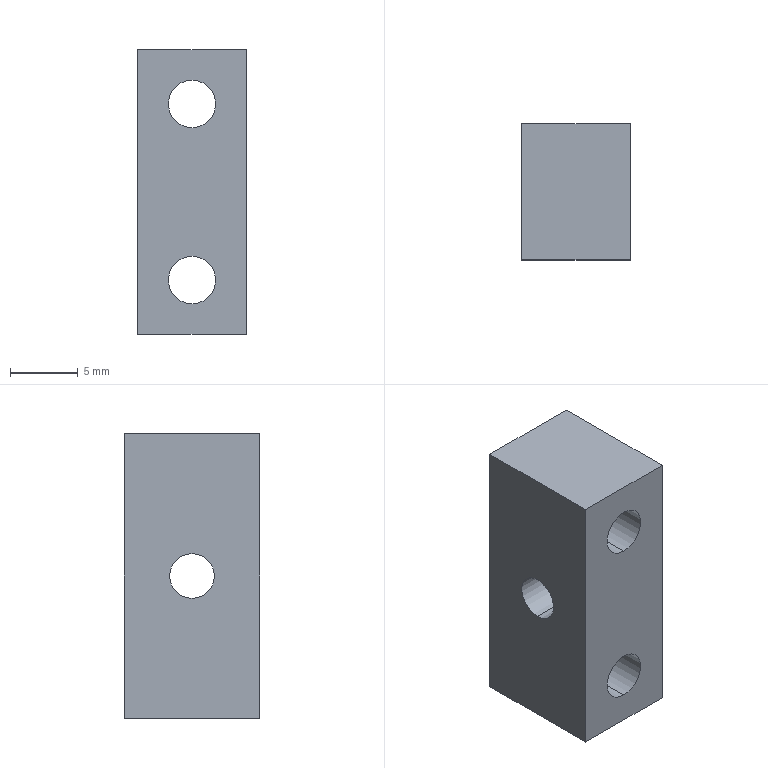Part | STEP file | 0246_211_Block | 1 solid | 18 faces | box 8 x 10 x 21 mm | volume 1254 mm3 | cylinder 10 | plane 8 | commonest cylinder face diameters 3.5 x4 6.5 x4 3.3 x2
STEP:
#1=CARTESIAN_POINT('',(0.,0.,0.));
#2=DIRECTION('',(0.,0.,1.));
#3=DIRECTION('',(1.,0.,0.));
#4=AXIS2_PLACEMENT_3D('',#1,#2,#3);
#5=CARTESIAN_POINT('',(0.,5.,-1.65));
#6=VERTEX_POINT('',#5);
#7=CARTESIAN_POINT('',(8.,5.,-1.65));
#8=VERTEX_POINT('',#7);
#9=CARTESIAN_POINT('',(8.,5.,-1.65));
#10=DIRECTION('',(1.,0.,0.));
#11=VECTOR('',#10,1.);
#12=LINE('',#9,#11);
#13=CARTESIAN_POINT('',(8.,5.,0.));
#14=DIRECTION('',(1.,0.,0.));
#15=DIRECTION('',(0.,0.,-1.));
#16=AXIS2_PLACEMENT_3D('',#13,#14,#15);
#17=CYLINDRICAL_SURFACE('',#16,1.65);
#18=CARTESIAN_POINT('',(6.283,0.));
#19=DIRECTION('',(0.,1.));
#20=VECTOR('',#19,1.);
#21=LINE('',#18,#20);
#22=(GEOMETRIC_REPRESENTATION_CONTEXT(2)PARAMETRIC_REPRESENTATION_CONTEXT()REPRESENTATION_CONTEXT('',''));
#23=DEFINITIONAL_REPRESENTATION('',(#21),#22);
#24=PCURVE('',#17,#23);
#25=CARTESIAN_POINT('',(8.,5.,0.));
#26=DIRECTION('',(1.,0.,0.));
#27=DIRECTION('',(0.,0.,-1.));
#28=AXIS2_PLACEMENT_3D('',#25,#26,#27);
#29=CYLINDRICAL_SURFACE('',#28,1.65);
#30=CARTESIAN_POINT('',(0.,0.));
#31=DIRECTION('',(0.,1.));
#32=VECTOR('',#31,1.);
#33=LINE('',#30,#32);
#34=(GEOMETRIC_REPRESENTATION_CONTEXT(2)PARAMETRIC_REPRESENTATION_CONTEXT()REPRESENTATION_CONTEXT('',''));
#35=DEFINITIONAL_REPRESENTATION('',(#33),#34);
#36=PCURVE('',#29,#35);
#37=SURFACE_CURVE('',#12,(#24,#36),.PCURVE_S1.);
#38=EDGE_CURVE('',#6,#8,#37,.T.);
#39=ORIENTED_EDGE('',*,*,#38,.T.);
#40=CARTESIAN_POINT('',(8.,5.,1.65));
#41=VERTEX_POINT('',#40);
#42=CARTESIAN_POINT('',(8.,5.,0.));
#43=DIRECTION('',(1.,0.,0.));
#44=DIRECTION('',(0.,0.,-1.));
#45=AXIS2_PLACEMENT_3D('',#42,#43,#44);
#46=CIRCLE('',#45,1.65);
#47=CARTESIAN_POINT('',(0.,0.));
#48=DIRECTION('',(1.,0.));
#49=VECTOR('',#48,1.);
#50=LINE('',#47,#49);
#51=(GEOMETRIC_REPRESENTATION_CONTEXT(2)PARAMETRIC_REPRESENTATION_CONTEXT()REPRESENTATION_CONTEXT('',''));
#52=DEFINITIONAL_REPRESENTATION('',(#50),#51);
#53=PCURVE('',#17,#52);
#54=CARTESIAN_POINT('',(8.,10.,-10.5));
#55=DIRECTION('',(-1.,0.,0.));
#56=DIRECTION('',(0.,0.,1.));
#57=AXIS2_PLACEMENT_3D('',#54,#55,#56);
#58=PLANE('',#57);
#59=CARTESIAN_POINT('',(8.85,-5.));
#60=CARTESIAN_POINT('',(8.85,-2.142));
#61=CARTESIAN_POINT('',(11.325,-3.571));
#62=CARTESIAN_POINT('',(13.8,-5.));
#63=CARTESIAN_POINT('',(11.325,-6.429));
#64=CARTESIAN_POINT('',(8.85,-7.858));
#65=CARTESIAN_POINT('',(8.85,-5.));
#66=(BOUNDED_CURVE()B_SPLINE_CURVE(2,(#59,#60,#61,#62,#63,#64,#65),.UNSPECIFIED.,.T.,.F.)B_SPLINE_CURVE_WITH_KNOTS((1,2,2,2,2,1),(-2.094,0.,2.094,4.189,6.283,8.378),.UNSPECIFIED.)CURVE()GEOMETRIC_REPRESENTATION_ITEM()RATIONAL_B_SPLINE_CURVE((1.,0.5,1.,0.5,1.,0.5,1.))REPRESENTATION_ITEM(''));
#67=(GEOMETRIC_REPRESENTATION_CONTEXT(2)PARAMETRIC_REPRESENTATION_CONTEXT()REPRESENTATION_CONTEXT('',''));
#68=DEFINITIONAL_REPRESENTATION('',(#66),#67);
#69=PCURVE('',#58,#68);
#70=SURFACE_CURVE('',#46,(#53,#69),.PCURVE_S1.);
#71=EDGE_CURVE('',#41,#8,#70,.T.);
#72=ORIENTED_EDGE('',*,*,#71,.F.);
#73=CARTESIAN_POINT('',(0.,5.,1.65));
#74=VERTEX_POINT('',#73);
#75=CARTESIAN_POINT('',(8.,5.,1.65));
#76=DIRECTION('',(1.,0.,0.));
#77=VECTOR('',#76,1.);
#78=LINE('',#75,#77);
#79=CARTESIAN_POINT('',(3.142,0.));
#80=DIRECTION('',(0.,1.));
#81=VECTOR('',#80,1.);
#82=LINE('',#79,#81);
#83=(GEOMETRIC_REPRESENTATION_CONTEXT(2)PARAMETRIC_REPRESENTATION_CONTEXT()REPRESENTATION_CONTEXT('',''));
#84=DEFINITIONAL_REPRESENTATION('',(#82),#83);
#85=PCURVE('',#17,#84);
#86=CARTESIAN_POINT('',(3.142,0.));
#87=DIRECTION('',(0.,1.));
#88=VECTOR('',#87,1.);
#89=LINE('',#86,#88);
#90=(GEOMETRIC_REPRESENTATION_CONTEXT(2)PARAMETRIC_REPRESENTATION_CONTEXT()REPRESENTATION_CONTEXT('',''));
#91=DEFINITIONAL_REPRESENTATION('',(#89),#90);
#92=PCURVE('',#29,#91);
#93=SURFACE_CURVE('',#78,(#85,#92),.PCURVE_S1.);
#94=EDGE_CURVE('',#74,#41,#93,.T.);
#95=ORIENTED_EDGE('',*,*,#94,.F.);
#96=CARTESIAN_POINT('',(0.,5.,0.));
#97=DIRECTION('',(1.,0.,0.));
#98=DIRECTION('',(0.,0.,-1.));
#99=AXIS2_PLACEMENT_3D('',#96,#97,#98);
#100=CIRCLE('',#99,1.65);
#101=CARTESIAN_POINT('',(0.,-8.));
#102=DIRECTION('',(1.,0.));
#103=VECTOR('',#102,1.);
#104=LINE('',#101,#103);
#105=(GEOMETRIC_REPRESENTATION_CONTEXT(2)PARAMETRIC_REPRESENTATION_CONTEXT()REPRESENTATION_CONTEXT('',''));
#106=DEFINITIONAL_REPRESENTATION('',(#104),#105);
#107=PCURVE('',#17,#106);
#108=CARTESIAN_POINT('',(0.,10.,-10.5));
#109=DIRECTION('',(1.,0.,0.));
#110=DIRECTION('',(0.,0.,-1.));
#111=AXIS2_PLACEMENT_3D('',#108,#109,#110);
#112=PLANE('',#111);
#113=CARTESIAN_POINT('',(-10.5,-5.));
#114=DIRECTION('',(1.,0.));
#115=AXIS2_PLACEMENT_2D('',#113,#114);
#116=CIRCLE('',#115,1.65);
#117=(GEOMETRIC_REPRESENTATION_CONTEXT(2)PARAMETRIC_REPRESENTATION_CONTEXT()REPRESENTATION_CONTEXT('',''));
#118=DEFINITIONAL_REPRESENTATION('',(#116),#117);
#119=PCURVE('',#112,#118);
#120=SURFACE_CURVE('',#100,(#107,#119),.PCURVE_S1.);
#121=EDGE_CURVE('',#74,#6,#120,.T.);
#122=ORIENTED_EDGE('',*,*,#121,.T.);
#123=EDGE_LOOP('',(#39,#72,#95,#122));
#124=FACE_BOUND('',#123,.F.);
#125=ADVANCED_FACE('',(#124),#17,.F.);
#126=CARTESIAN_POINT('',(4.,6.5,9.75));
#127=VERTEX_POINT('',#126);
#128=CARTESIAN_POINT('',(4.,10.,9.75));
#129=VERTEX_POINT('',#128);
#130=CARTESIAN_POINT('',(4.,10.,9.75));
#131=DIRECTION('',(0.,1.,0.));
#132=VECTOR('',#131,1.);
#133=LINE('',#130,#132);
#134=CARTESIAN_POINT('',(4.,10.,6.5));
#135=DIRECTION('',(0.,1.,0.));
#136=DIRECTION('',(0.,0.,1.));
#137=AXIS2_PLACEMENT_3D('',#134,#135,#136);
#138=CYLINDRICAL_SURFACE('',#137,3.25);
#139=CARTESIAN_POINT('',(6.283,0.));
#140=DIRECTION('',(0.,1.));
#141=VECTOR('',#140,1.);
#142=LINE('',#139,#141);
#143=(GEOMETRIC_REPRESENTATION_CONTEXT(2)PARAMETRIC_REPRESENTATION_CONTEXT()REPRESENTATION_CONTEXT('',''));
#144=DEFINITIONAL_REPRESENTATION('',(#142),#143);
#145=PCURVE('',#138,#144);
#146=CARTESIAN_POINT('',(4.,10.,6.5));
#147=DIRECTION('',(0.,1.,0.));
#148=DIRECTION('',(0.,0.,1.));
#149=AXIS2_PLACEMENT_3D('',#146,#147,#148);
#150=CYLINDRICAL_SURFACE('',#149,3.25);
#151=CARTESIAN_POINT('',(0.,0.));
#152=DIRECTION('',(0.,1.));
#153=VECTOR('',#152,1.);
#154=LINE('',#151,#153);
#155=(GEOMETRIC_REPRESENTATION_CONTEXT(2)PARAMETRIC_REPRESENTATION_CONTEXT()REPRESENTATION_CONTEXT('',''));
#156=DEFINITIONAL_REPRESENTATION('',(#154),#155);
#157=PCURVE('',#150,#156);
#158=SURFACE_CURVE('',#133,(#145,#157),.PCURVE_S1.);
#159=EDGE_CURVE('',#127,#129,#158,.T.);
#160=ORIENTED_EDGE('',*,*,#159,.T.);
#161=CARTESIAN_POINT('',(4.,10.,3.25));
#162=VERTEX_POINT('',#161);
#163=CARTESIAN_POINT('',(4.,10.,6.5));
#164=DIRECTION('',(0.,1.,0.));
#165=DIRECTION('',(0.,0.,1.));
#166=AXIS2_PLACEMENT_3D('',#163,#164,#165);
#167=CIRCLE('',#166,3.25);
#168=CARTESIAN_POINT('',(0.,0.));
#169=DIRECTION('',(1.,0.));
#170=VECTOR('',#169,1.);
#171=LINE('',#168,#170);
#172=(GEOMETRIC_REPRESENTATION_CONTEXT(2)PARAMETRIC_REPRESENTATION_CONTEXT()REPRESENTATION_CONTEXT('',''));
#173=DEFINITIONAL_REPRESENTATION('',(#171),#172);
#174=PCURVE('',#138,#173);
#175=CARTESIAN_POINT('',(0.,10.,10.5));
#176=DIRECTION('',(0.,1.,0.));
#177=DIRECTION('',(0.,0.,1.));
#178=AXIS2_PLACEMENT_3D('',#175,#176,#177);
#179=PLANE('',#178);
#180=CARTESIAN_POINT('',(-4.,4.));
#181=DIRECTION('',(1.,0.));
#182=AXIS2_PLACEMENT_2D('',#180,#181);
#183=CIRCLE('',#182,3.25);
#184=(GEOMETRIC_REPRESENTATION_CONTEXT(2)PARAMETRIC_REPRESENTATION_CONTEXT()REPRESENTATION_CONTEXT('',''));
#185=DEFINITIONAL_REPRESENTATION('',(#183),#184);
#186=PCURVE('',#179,#185);
#187=SURFACE_CURVE('',#167,(#174,#186),.PCURVE_S1.);
#188=EDGE_CURVE('',#162,#129,#187,.T.);
#189=ORIENTED_EDGE('',*,*,#188,.F.);
#190=CARTESIAN_POINT('',(4.,6.5,3.25));
#191=VERTEX_POINT('',#190);
#192=CARTESIAN_POINT('',(4.,10.,3.25));
#193=DIRECTION('',(0.,1.,0.));
#194=VECTOR('',#193,1.);
#195=LINE('',#192,#194);
#196=CARTESIAN_POINT('',(3.142,0.));
#197=DIRECTION('',(0.,1.));
#198=VECTOR('',#197,1.);
#199=LINE('',#196,#198);
#200=(GEOMETRIC_REPRESENTATION_CONTEXT(2)PARAMETRIC_REPRESENTATION_CONTEXT()REPRESENTATION_CONTEXT('',''));
#201=DEFINITIONAL_REPRESENTATION('',(#199),#200);
#202=PCURVE('',#138,#201);
#203=CARTESIAN_POINT('',(3.142,0.));
#204=DIRECTION('',(0.,1.));
#205=VECTOR('',#204,1.);
#206=LINE('',#203,#205);
#207=(GEOMETRIC_REPRESENTATION_CONTEXT(2)PARAMETRIC_REPRESENTATION_CONTEXT()REPRESENTATION_CONTEXT('',''));
#208=DEFINITIONAL_REPRESENTATION('',(#206),#207);
#209=PCURVE('',#150,#208);
#210=SURFACE_CURVE('',#195,(#202,#209),.PCURVE_S1.);
#211=EDGE_CURVE('',#191,#162,#210,.T.);
#212=ORIENTED_EDGE('',*,*,#211,.F.);
#213=CARTESIAN_POINT('',(4.,6.5,6.5));
#214=DIRECTION('',(0.,1.,0.));
#215=DIRECTION('',(0.,0.,1.));
#216=AXIS2_PLACEMENT_3D('',#213,#214,#215);
#217=CIRCLE('',#216,3.25);
#218=CARTESIAN_POINT('',(0.,-3.5));
#219=DIRECTION('',(1.,0.));
#220=VECTOR('',#219,1.);
#221=LINE('',#218,#220);
#222=(GEOMETRIC_REPRESENTATION_CONTEXT(2)PARAMETRIC_REPRESENTATION_CONTEXT()REPRESENTATION_CONTEXT('',''));
#223=DEFINITIONAL_REPRESENTATION('',(#221),#222);
#224=PCURVE('',#138,#223);
#225=CARTESIAN_POINT('',(5.75,6.5,6.5));
#226=DIRECTION('',(0.,-1.,0.));
#227=DIRECTION('',(0.,0.,-1.));
#228=AXIS2_PLACEMENT_3D('',#225,#226,#227);
#229=PLANE('',#228);
#230=CARTESIAN_POINT('',(-3.25,-1.75));
#231=CARTESIAN_POINT('',(-3.25,3.879));
#232=CARTESIAN_POINT('',(1.625,1.065));
#233=CARTESIAN_POINT('',(6.5,-1.75));
#234=CARTESIAN_POINT('',(1.625,-4.565));
#235=CARTESIAN_POINT('',(-3.25,-7.379));
#236=CARTESIAN_POINT('',(-3.25,-1.75));
#237=(BOUNDED_CURVE()B_SPLINE_CURVE(2,(#230,#231,#232,#233,#234,#235,#236),.UNSPECIFIED.,.T.,.F.)B_SPLINE_CURVE_WITH_KNOTS((1,2,2,2,2,1),(-2.094,0.,2.094,4.189,6.283,8.378),.UNSPECIFIED.)CURVE()GEOMETRIC_REPRESENTATION_ITEM()RATIONAL_B_SPLINE_CURVE((1.,0.5,1.,0.5,1.,0.5,1.))REPRESENTATION_ITEM(''));
#238=(GEOMETRIC_REPRESENTATION_CONTEXT(2)PARAMETRIC_REPRESENTATION_CONTEXT()REPRESENTATION_CONTEXT('',''));
#239=DEFINITIONAL_REPRESENTATION('',(#237),#238);
#240=PCURVE('',#229,#239);
#241=SURFACE_CURVE('',#217,(#224,#240),.PCURVE_S1.);
#242=EDGE_CURVE('',#191,#127,#241,.T.);
#243=ORIENTED_EDGE('',*,*,#242,.T.);
#244=EDGE_LOOP('',(#160,#189,#212,#243));
#245=FACE_BOUND('',#244,.F.);
#246=ADVANCED_FACE('',(#245),#138,.F.);
#247=CARTESIAN_POINT('',(4.,0.,8.25));
#248=VERTEX_POINT('',#247);
#249=CARTESIAN_POINT('',(4.,6.5,8.25));
#250=VERTEX_POINT('',#249);
#251=CARTESIAN_POINT('',(4.,10.,8.25));
#252=DIRECTION('',(0.,1.,0.));
#253=VECTOR('',#252,1.);
#254=LINE('',#251,#253);
#255=CARTESIAN_POINT('',(4.,10.,6.5));
#256=DIRECTION('',(0.,1.,0.));
#257=DIRECTION('',(0.,0.,1.));
#258=AXIS2_PLACEMENT_3D('',#255,#256,#257);
#259=CYLINDRICAL_SURFACE('',#258,1.75);
#260=CARTESIAN_POINT('',(6.283,0.));
#261=DIRECTION('',(0.,1.));
#262=VECTOR('',#261,1.);
#263=LINE('',#260,#262);
#264=(GEOMETRIC_REPRESENTATION_CONTEXT(2)PARAMETRIC_REPRESENTATION_CONTEXT()REPRESENTATION_CONTEXT('',''));
#265=DEFINITIONAL_REPRESENTATION('',(#263),#264);
#266=PCURVE('',#259,#265);
#267=CARTESIAN_POINT('',(4.,10.,6.5));
#268=DIRECTION('',(0.,1.,0.));
#269=DIRECTION('',(0.,0.,1.));
#270=AXIS2_PLACEMENT_3D('',#267,#268,#269);
#271=CYLINDRICAL_SURFACE('',#270,1.75);
#272=CARTESIAN_POINT('',(0.,0.));
#273=DIRECTION('',(0.,1.));
#274=VECTOR('',#273,1.);
#275=LINE('',#272,#274);
#276=(GEOMETRIC_REPRESENTATION_CONTEXT(2)PARAMETRIC_REPRESENTATION_CONTEXT()REPRESENTATION_CONTEXT('',''));
#277=DEFINITIONAL_REPRESENTATION('',(#275),#276);
#278=PCURVE('',#271,#277);
#279=SURFACE_CURVE('',#254,(#266,#278),.PCURVE_S1.);
#280=EDGE_CURVE('',#248,#250,#279,.T.);
#281=ORIENTED_EDGE('',*,*,#280,.T.);
#282=CARTESIAN_POINT('',(4.,6.5,4.75));
#283=VERTEX_POINT('',#282);
#284=CARTESIAN_POINT('',(4.,6.5,6.5));
#285=DIRECTION('',(0.,1.,0.));
#286=DIRECTION('',(0.,0.,1.));
#287=AXIS2_PLACEMENT_3D('',#284,#285,#286);
#288=CIRCLE('',#287,1.75);
#289=CARTESIAN_POINT('',(0.,-3.5));
#290=DIRECTION('',(1.,0.));
#291=VECTOR('',#290,1.);
#292=LINE('',#289,#291);
#293=(GEOMETRIC_REPRESENTATION_CONTEXT(2)PARAMETRIC_REPRESENTATION_CONTEXT()REPRESENTATION_CONTEXT('',''));
#294=DEFINITIONAL_REPRESENTATION('',(#292),#293);
#295=PCURVE('',#259,#294);
#296=CARTESIAN_POINT('',(-1.75,-1.75));
#297=CARTESIAN_POINT('',(-1.75,1.281));
#298=CARTESIAN_POINT('',(0.875,-0.2345));
#299=CARTESIAN_POINT('',(3.5,-1.75));
#300=CARTESIAN_POINT('',(0.875,-3.266));
#301=CARTESIAN_POINT('',(-1.75,-4.781));
#302=CARTESIAN_POINT('',(-1.75,-1.75));
#303=(BOUNDED_CURVE()B_SPLINE_CURVE(2,(#296,#297,#298,#299,#300,#301,#302),.UNSPECIFIED.,.T.,.F.)B_SPLINE_CURVE_WITH_KNOTS((1,2,2,2,2,1),(-2.094,0.,2.094,4.189,6.283,8.378),.UNSPECIFIED.)CURVE()GEOMETRIC_REPRESENTATION_ITEM()RATIONAL_B_SPLINE_CURVE((1.,0.5,1.,0.5,1.,0.5,1.))REPRESENTATION_ITEM(''));
#304=(GEOMETRIC_REPRESENTATION_CONTEXT(2)PARAMETRIC_REPRESENTATION_CONTEXT()REPRESENTATION_CONTEXT('',''));
#305=DEFINITIONAL_REPRESENTATION('',(#303),#304);
#306=PCURVE('',#229,#305);
#307=SURFACE_CURVE('',#288,(#295,#306),.PCURVE_S1.);
#308=EDGE_CURVE('',#283,#250,#307,.T.);
#309=ORIENTED_EDGE('',*,*,#308,.F.);
#310=CARTESIAN_POINT('',(4.,0.,4.75));
#311=VERTEX_POINT('',#310);
#312=CARTESIAN_POINT('',(4.,10.,4.75));
#313=DIRECTION('',(0.,1.,0.));
#314=VECTOR('',#313,1.);
#315=LINE('',#312,#314);
#316=CARTESIAN_POINT('',(3.142,0.));
#317=DIRECTION('',(0.,1.));
#318=VECTOR('',#317,1.);
#319=LINE('',#316,#318);
#320=(GEOMETRIC_REPRESENTATION_CONTEXT(2)PARAMETRIC_REPRESENTATION_CONTEXT()REPRESENTATION_CONTEXT('',''));
#321=DEFINITIONAL_REPRESENTATION('',(#319),#320);
#322=PCURVE('',#259,#321);
#323=CARTESIAN_POINT('',(3.142,0.));
#324=DIRECTION('',(0.,1.));
#325=VECTOR('',#324,1.);
#326=LINE('',#323,#325);
#327=(GEOMETRIC_REPRESENTATION_CONTEXT(2)PARAMETRIC_REPRESENTATION_CONTEXT()REPRESENTATION_CONTEXT('',''));
#328=DEFINITIONAL_REPRESENTATION('',(#326),#327);
#329=PCURVE('',#271,#328);
#330=SURFACE_CURVE('',#315,(#322,#329),.PCURVE_S1.);
#331=EDGE_CURVE('',#311,#283,#330,.T.);
#332=ORIENTED_EDGE('',*,*,#331,.F.);
#333=CARTESIAN_POINT('',(4.,0.,6.5));
#334=DIRECTION('',(0.,1.,0.));
#335=DIRECTION('',(0.,0.,1.));
#336=AXIS2_PLACEMENT_3D('',#333,#334,#335);
#337=CIRCLE('',#336,1.75);
#338=CARTESIAN_POINT('',(0.,-10.));
#339=DIRECTION('',(1.,0.));
#340=VECTOR('',#339,1.);
#341=LINE('',#338,#340);
#342=(GEOMETRIC_REPRESENTATION_CONTEXT(2)PARAMETRIC_REPRESENTATION_CONTEXT()REPRESENTATION_CONTEXT('',''));
#343=DEFINITIONAL_REPRESENTATION('',(#341),#342);
#344=PCURVE('',#259,#343);
#345=CARTESIAN_POINT('',(0.,0.,10.5));
#346=DIRECTION('',(0.,1.,0.));
#347=DIRECTION('',(0.,0.,1.));
#348=AXIS2_PLACEMENT_3D('',#345,#346,#347);
#349=PLANE('',#348);
#350=CARTESIAN_POINT('',(-4.,4.));
#351=DIRECTION('',(1.,0.));
#352=AXIS2_PLACEMENT_2D('',#350,#351);
#353=CIRCLE('',#352,1.75);
#354=(GEOMETRIC_REPRESENTATION_CONTEXT(2)PARAMETRIC_REPRESENTATION_CONTEXT()REPRESENTATION_CONTEXT('',''));
#355=DEFINITIONAL_REPRESENTATION('',(#353),#354);
#356=PCURVE('',#349,#355);
#357=SURFACE_CURVE('',#337,(#344,#356),.PCURVE_S1.);
#358=EDGE_CURVE('',#311,#248,#357,.T.);
#359=ORIENTED_EDGE('',*,*,#358,.T.);
#360=EDGE_LOOP('',(#281,#309,#332,#359));
#361=FACE_BOUND('',#360,.F.);
#362=ADVANCED_FACE('',(#361),#259,.F.);
#363=CARTESIAN_POINT('',(4.,6.5,-3.25));
#364=VERTEX_POINT('',#363);
#365=CARTESIAN_POINT('',(4.,10.,-3.25));
#366=VERTEX_POINT('',#365);
#367=CARTESIAN_POINT('',(4.,10.,-3.25));
#368=DIRECTION('',(0.,1.,0.));
#369=VECTOR('',#368,1.);
#370=LINE('',#367,#369);
#371=CARTESIAN_POINT('',(4.,10.,-6.5));
#372=DIRECTION('',(0.,1.,0.));
#373=DIRECTION('',(0.,0.,1.));
#374=AXIS2_PLACEMENT_3D('',#371,#372,#373);
#375=CYLINDRICAL_SURFACE('',#374,3.25);
#376=CARTESIAN_POINT('',(6.283,0.));
#377=DIRECTION('',(0.,1.));
#378=VECTOR('',#377,1.);
#379=LINE('',#376,#378);
#380=(GEOMETRIC_REPRESENTATION_CONTEXT(2)PARAMETRIC_REPRESENTATION_CONTEXT()REPRESENTATION_CONTEXT('',''));
#381=DEFINITIONAL_REPRESENTATION('',(#379),#380);
#382=PCURVE('',#375,#381);
#383=CARTESIAN_POINT('',(4.,10.,-6.5));
#384=DIRECTION('',(0.,1.,0.));
#385=DIRECTION('',(0.,0.,1.));
#386=AXIS2_PLACEMENT_3D('',#383,#384,#385);
#387=CYLINDRICAL_SURFACE('',#386,3.25);
#388=CARTESIAN_POINT('',(0.,0.));
#389=DIRECTION('',(0.,1.));
#390=VECTOR('',#389,1.);
#391=LINE('',#388,#390);
#392=(GEOMETRIC_REPRESENTATION_CONTEXT(2)PARAMETRIC_REPRESENTATION_CONTEXT()REPRESENTATION_CONTEXT('',''));
#393=DEFINITIONAL_REPRESENTATION('',(#391),#392);
#394=PCURVE('',#387,#393);
#395=SURFACE_CURVE('',#370,(#382,#394),.PCURVE_S1.);
#396=EDGE_CURVE('',#364,#366,#395,.T.);
#397=ORIENTED_EDGE('',*,*,#396,.T.);
#398=CARTESIAN_POINT('',(4.,10.,-9.75));
#399=VERTEX_POINT('',#398);
#400=CARTESIAN_POINT('',(4.,10.,-6.5));
#401=DIRECTION('',(0.,1.,0.));
#402=DIRECTION('',(0.,0.,1.));
#403=AXIS2_PLACEMENT_3D('',#400,#401,#402);
#404=CIRCLE('',#403,3.25);
#405=CARTESIAN_POINT('',(0.,0.));
#406=DIRECTION('',(1.,0.));
#407=VECTOR('',#406,1.);
#408=LINE('',#405,#407);
#409=(GEOMETRIC_REPRESENTATION_CONTEXT(2)PARAMETRIC_REPRESENTATION_CONTEXT()REPRESENTATION_CONTEXT('',''));
#410=DEFINITIONAL_REPRESENTATION('',(#408),#409);
#411=PCURVE('',#375,#410);
#412=CARTESIAN_POINT('',(-17.,4.));
#413=DIRECTION('',(1.,0.));
#414=AXIS2_PLACEMENT_2D('',#412,#413);
#415=CIRCLE('',#414,3.25);
#416=(GEOMETRIC_REPRESENTATION_CONTEXT(2)PARAMETRIC_REPRESENTATION_CONTEXT()REPRESENTATION_CONTEXT('',''));
#417=DEFINITIONAL_REPRESENTATION('',(#415),#416);
#418=PCURVE('',#179,#417);
#419=SURFACE_CURVE('',#404,(#411,#418),.PCURVE_S1.);
#420=EDGE_CURVE('',#399,#366,#419,.T.);
#421=ORIENTED_EDGE('',*,*,#420,.F.);
#422=CARTESIAN_POINT('',(4.,6.5,-9.75));
#423=VERTEX_POINT('',#422);
#424=CARTESIAN_POINT('',(4.,10.,-9.75));
#425=DIRECTION('',(0.,1.,0.));
#426=VECTOR('',#425,1.);
#427=LINE('',#424,#426);
#428=CARTESIAN_POINT('',(3.142,0.));
#429=DIRECTION('',(0.,1.));
#430=VECTOR('',#429,1.);
#431=LINE('',#428,#430);
#432=(GEOMETRIC_REPRESENTATION_CONTEXT(2)PARAMETRIC_REPRESENTATION_CONTEXT()REPRESENTATION_CONTEXT('',''));
#433=DEFINITIONAL_REPRESENTATION('',(#431),#432);
#434=PCURVE('',#375,#433);
#435=CARTESIAN_POINT('',(3.142,0.));
#436=DIRECTION('',(0.,1.));
#437=VECTOR('',#436,1.);
#438=LINE('',#435,#437);
#439=(GEOMETRIC_REPRESENTATION_CONTEXT(2)PARAMETRIC_REPRESENTATION_CONTEXT()REPRESENTATION_CONTEXT('',''));
#440=DEFINITIONAL_REPRESENTATION('',(#438),#439);
#441=PCURVE('',#387,#440);
#442=SURFACE_CURVE('',#427,(#434,#441),.PCURVE_S1.);
#443=EDGE_CURVE('',#423,#399,#442,.T.);
#444=ORIENTED_EDGE('',*,*,#443,.F.);
#445=CARTESIAN_POINT('',(4.,6.5,-6.5));
#446=DIRECTION('',(0.,1.,0.));
#447=DIRECTION('',(0.,0.,1.));
#448=AXIS2_PLACEMENT_3D('',#445,#446,#447);
#449=CIRCLE('',#448,3.25);
#450=CARTESIAN_POINT('',(0.,-3.5));
#451=DIRECTION('',(1.,0.));
#452=VECTOR('',#451,1.);
#453=LINE('',#450,#452);
#454=(GEOMETRIC_REPRESENTATION_CONTEXT(2)PARAMETRIC_REPRESENTATION_CONTEXT()REPRESENTATION_CONTEXT('',''));
#455=DEFINITIONAL_REPRESENTATION('',(#453),#454);
#456=PCURVE('',#375,#455);
#457=CARTESIAN_POINT('',(5.75,6.5,-6.5));
#458=DIRECTION('',(0.,-1.,0.));
#459=DIRECTION('',(0.,0.,-1.));
#460=AXIS2_PLACEMENT_3D('',#457,#458,#459);
#461=PLANE('',#460);
#462=CARTESIAN_POINT('',(-3.25,-1.75));
#463=CARTESIAN_POINT('',(-3.25,3.879));
#464=CARTESIAN_POINT('',(1.625,1.065));
#465=CARTESIAN_POINT('',(6.5,-1.75));
#466=CARTESIAN_POINT('',(1.625,-4.565));
#467=CARTESIAN_POINT('',(-3.25,-7.379));
#468=CARTESIAN_POINT('',(-3.25,-1.75));
#469=(BOUNDED_CURVE()B_SPLINE_CURVE(2,(#462,#463,#464,#465,#466,#467,#468),.UNSPECIFIED.,.T.,.F.)B_SPLINE_CURVE_WITH_KNOTS((1,2,2,2,2,1),(-2.094,0.,2.094,4.189,6.283,8.378),.UNSPECIFIED.)CURVE()GEOMETRIC_REPRESENTATION_ITEM()RATIONAL_B_SPLINE_CURVE((1.,0.5,1.,0.5,1.,0.5,1.))REPRESENTATION_ITEM(''));
#470=(GEOMETRIC_REPRESENTATION_CONTEXT(2)PARAMETRIC_REPRESENTATION_CONTEXT()REPRESENTATION_CONTEXT('',''));
#471=DEFINITIONAL_REPRESENTATION('',(#469),#470);
#472=PCURVE('',#461,#471);
#473=SURFACE_CURVE('',#449,(#456,#472),.PCURVE_S1.);
#474=EDGE_CURVE('',#423,#364,#473,.T.);
#475=ORIENTED_EDGE('',*,*,#474,.T.);
#476=EDGE_LOOP('',(#397,#421,#444,#475));
#477=FACE_BOUND('',#476,.F.);
#478=ADVANCED_FACE('',(#477),#375,.F.);
#479=CARTESIAN_POINT('',(4.,0.,-4.75));
#480=VERTEX_POINT('',#479);
#481=CARTESIAN_POINT('',(4.,6.5,-4.75));
#482=VERTEX_POINT('',#481);
#483=CARTESIAN_POINT('',(4.,10.,-4.75));
#484=DIRECTION('',(0.,1.,0.));
#485=VECTOR('',#484,1.);
#486=LINE('',#483,#485);
#487=CARTESIAN_POINT('',(4.,10.,-6.5));
#488=DIRECTION('',(0.,1.,0.));
#489=DIRECTION('',(0.,0.,1.));
#490=AXIS2_PLACEMENT_3D('',#487,#488,#489);
#491=CYLINDRICAL_SURFACE('',#490,1.75);
#492=CARTESIAN_POINT('',(6.283,0.));
#493=DIRECTION('',(0.,1.));
#494=VECTOR('',#493,1.);
#495=LINE('',#492,#494);
#496=(GEOMETRIC_REPRESENTATION_CONTEXT(2)PARAMETRIC_REPRESENTATION_CONTEXT()REPRESENTATION_CONTEXT('',''));
#497=DEFINITIONAL_REPRESENTATION('',(#495),#496);
#498=PCURVE('',#491,#497);
#499=CARTESIAN_POINT('',(4.,10.,-6.5));
#500=DIRECTION('',(0.,1.,0.));
#501=DIRECTION('',(0.,0.,1.));
#502=AXIS2_PLACEMENT_3D('',#499,#500,#501);
#503=CYLINDRICAL_SURFACE('',#502,1.75);
#504=CARTESIAN_POINT('',(0.,0.));
#505=DIRECTION('',(0.,1.));
#506=VECTOR('',#505,1.);
#507=LINE('',#504,#506);
#508=(GEOMETRIC_REPRESENTATION_CONTEXT(2)PARAMETRIC_REPRESENTATION_CONTEXT()REPRESENTATION_CONTEXT('',''));
#509=DEFINITIONAL_REPRESENTATION('',(#507),#508);
#510=PCURVE('',#503,#509);
#511=SURFACE_CURVE('',#486,(#498,#510),.PCURVE_S1.);
#512=EDGE_CURVE('',#480,#482,#511,.T.);
#513=ORIENTED_EDGE('',*,*,#512,.T.);
#514=CARTESIAN_POINT('',(4.,6.5,-8.25));
#515=VERTEX_POINT('',#514);
#516=CARTESIAN_POINT('',(4.,6.5,-6.5));
#517=DIRECTION('',(0.,1.,0.));
#518=DIRECTION('',(0.,0.,1.));
#519=AXIS2_PLACEMENT_3D('',#516,#517,#518);
#520=CIRCLE('',#519,1.75);
#521=CARTESIAN_POINT('',(0.,-3.5));
#522=DIRECTION('',(1.,0.));
#523=VECTOR('',#522,1.);
#524=LINE('',#521,#523);
#525=(GEOMETRIC_REPRESENTATION_CONTEXT(2)PARAMETRIC_REPRESENTATION_CONTEXT()REPRESENTATION_CONTEXT('',''));
#526=DEFINITIONAL_REPRESENTATION('',(#524),#525);
#527=PCURVE('',#491,#526);
#528=CARTESIAN_POINT('',(-1.75,-1.75));
#529=CARTESIAN_POINT('',(-1.75,1.281));
#530=CARTESIAN_POINT('',(0.875,-0.2345));
#531=CARTESIAN_POINT('',(3.5,-1.75));
#532=CARTESIAN_POINT('',(0.875,-3.266));
#533=CARTESIAN_POINT('',(-1.75,-4.781));
#534=CARTESIAN_POINT('',(-1.75,-1.75));
#535=(BOUNDED_CURVE()B_SPLINE_CURVE(2,(#528,#529,#530,#531,#532,#533,#534),.UNSPECIFIED.,.T.,.F.)B_SPLINE_CURVE_WITH_KNOTS((1,2,2,2,2,1),(-2.094,0.,2.094,4.189,6.283,8.378),.UNSPECIFIED.)CURVE()GEOMETRIC_REPRESENTATION_ITEM()RATIONAL_B_SPLINE_CURVE((1.,0.5,1.,0.5,1.,0.5,1.))REPRESENTATION_ITEM(''));
#536=(GEOMETRIC_REPRESENTATION_CONTEXT(2)PARAMETRIC_REPRESENTATION_CONTEXT()REPRESENTATION_CONTEXT('',''));
#537=DEFINITIONAL_REPRESENTATION('',(#535),#536);
#538=PCURVE('',#461,#537);
#539=SURFACE_CURVE('',#520,(#527,#538),.PCURVE_S1.);
#540=EDGE_CURVE('',#515,#482,#539,.T.);
#541=ORIENTED_EDGE('',*,*,#540,.F.);
#542=CARTESIAN_POINT('',(4.,0.,-8.25));
#543=VERTEX_POINT('',#542);
#544=CARTESIAN_POINT('',(4.,10.,-8.25));
#545=DIRECTION('',(0.,1.,0.));
#546=VECTOR('',#545,1.);
#547=LINE('',#544,#546);
#548=CARTESIAN_POINT('',(3.142,0.));
#549=DIRECTION('',(0.,1.));
#550=VECTOR('',#549,1.);
#551=LINE('',#548,#550);
#552=(GEOMETRIC_REPRESENTATION_CONTEXT(2)PARAMETRIC_REPRESENTATION_CONTEXT()REPRESENTATION_CONTEXT('',''));
#553=DEFINITIONAL_REPRESENTATION('',(#551),#552);
#554=PCURVE('',#491,#553);
#555=CARTESIAN_POINT('',(3.142,0.));
#556=DIRECTION('',(0.,1.));
#557=VECTOR('',#556,1.);
#558=LINE('',#555,#557);
#559=(GEOMETRIC_REPRESENTATION_CONTEXT(2)PARAMETRIC_REPRESENTATION_CONTEXT()REPRESENTATION_CONTEXT('',''));
#560=DEFINITIONAL_REPRESENTATION('',(#558),#559);
#561=PCURVE('',#503,#560);
#562=SURFACE_CURVE('',#547,(#554,#561),.PCURVE_S1.);
#563=EDGE_CURVE('',#543,#515,#562,.T.);
#564=ORIENTED_EDGE('',*,*,#563,.F.);
#565=CARTESIAN_POINT('',(4.,0.,-6.5));
#566=DIRECTION('',(0.,1.,0.));
#567=DIRECTION('',(0.,0.,1.));
#568=AXIS2_PLACEMENT_3D('',#565,#566,#567);
#569=CIRCLE('',#568,1.75);
#570=CARTESIAN_POINT('',(0.,-10.));
#571=DIRECTION('',(1.,0.));
#572=VECTOR('',#571,1.);
#573=LINE('',#570,#572);
#574=(GEOMETRIC_REPRESENTATION_CONTEXT(2)PARAMETRIC_REPRESENTATION_CONTEXT()REPRESENTATION_CONTEXT('',''));
#575=DEFINITIONAL_REPRESENTATION('',(#573),#574);
#576=PCURVE('',#491,#575);
#577=CARTESIAN_POINT('',(-17.,4.));
#578=DIRECTION('',(1.,0.));
#579=AXIS2_PLACEMENT_2D('',#577,#578);
#580=CIRCLE('',#579,1.75);
#581=(GEOMETRIC_REPRESENTATION_CONTEXT(2)PARAMETRIC_REPRESENTATION_CONTEXT()REPRESENTATION_CONTEXT('',''));
#582=DEFINITIONAL_REPRESENTATION('',(#580),#581);
#583=PCURVE('',#349,#582);
#584=SURFACE_CURVE('',#569,(#576,#583),.PCURVE_S1.);
#585=EDGE_CURVE('',#543,#480,#584,.T.);
#586=ORIENTED_EDGE('',*,*,#585,.T.);
#587=EDGE_LOOP('',(#513,#541,#564,#586));
#588=FACE_BOUND('',#587,.F.);
#589=ADVANCED_FACE('',(#588),#491,.F.);
#590=CARTESIAN_POINT('',(0.,5.,0.));
#591=DIRECTION('',(1.,0.,0.));
#592=DIRECTION('',(0.,0.,-1.));
#593=AXIS2_PLACEMENT_3D('',#590,#591,#592);
#594=CIRCLE('',#593,1.65);
#595=CARTESIAN_POINT('',(-10.5,-5.));
#596=DIRECTION('',(1.,0.));
#597=AXIS2_PLACEMENT_2D('',#595,#596);
#598=CIRCLE('',#597,1.65);
#599=(GEOMETRIC_REPRESENTATION_CONTEXT(2)PARAMETRIC_REPRESENTATION_CONTEXT()REPRESENTATION_CONTEXT('',''));
#600=DEFINITIONAL_REPRESENTATION('',(#598),#599);
#601=PCURVE('',#112,#600);
#602=CARTESIAN_POINT('',(0.,-8.));
#603=DIRECTION('',(1.,0.));
#604=VECTOR('',#603,1.);
#605=LINE('',#602,#604);
#606=(GEOMETRIC_REPRESENTATION_CONTEXT(2)PARAMETRIC_REPRESENTATION_CONTEXT()REPRESENTATION_CONTEXT('',''));
#607=DEFINITIONAL_REPRESENTATION('',(#605),#606);
#608=PCURVE('',#29,#607);
#609=SURFACE_CURVE('',#594,(#601,#608),.PCURVE_S1.);
#610=EDGE_CURVE('',#6,#74,#609,.T.);
#611=ORIENTED_EDGE('',*,*,#610,.T.);
#612=ORIENTED_EDGE('',*,*,#121,.T.);
#613=EDGE_LOOP('',(#611,#612));
#614=FACE_BOUND('',#613,.T.);
#615=CARTESIAN_POINT('',(0.,0.,-10.5));
#616=VERTEX_POINT('',#615);
#617=CARTESIAN_POINT('',(0.,0.,10.5));
#618=VERTEX_POINT('',#617);
#619=CARTESIAN_POINT('',(0.,0.,-10.5));
#620=DIRECTION('',(0.,0.,1.));
#621=VECTOR('',#620,1.);
#622=LINE('',#619,#621);
#623=CARTESIAN_POINT('',(0.,-10.));
#624=DIRECTION('',(-1.,0.));
#625=VECTOR('',#624,1.);
#626=LINE('',#623,#625);
#627=(GEOMETRIC_REPRESENTATION_CONTEXT(2)PARAMETRIC_REPRESENTATION_CONTEXT()REPRESENTATION_CONTEXT('',''));
#628=DEFINITIONAL_REPRESENTATION('',(#626),#627);
#629=PCURVE('',#112,#628);
#630=CARTESIAN_POINT('',(-21.,0.));
#631=DIRECTION('',(1.,0.));
#632=VECTOR('',#631,1.);
#633=LINE('',#630,#632);
#634=(GEOMETRIC_REPRESENTATION_CONTEXT(2)PARAMETRIC_REPRESENTATION_CONTEXT()REPRESENTATION_CONTEXT('',''));
#635=DEFINITIONAL_REPRESENTATION('',(#633),#634);
#636=PCURVE('',#349,#635);
#637=SURFACE_CURVE('',#622,(#629,#636),.PCURVE_S1.);
#638=EDGE_CURVE('',#616,#618,#637,.T.);
#639=ORIENTED_EDGE('',*,*,#638,.T.);
#640=CARTESIAN_POINT('',(0.,10.,10.5));
#641=VERTEX_POINT('',#640);
#642=CARTESIAN_POINT('',(0.,10.,10.5));
#643=DIRECTION('',(0.,-1.,0.));
#644=VECTOR('',#643,1.);
#645=LINE('',#642,#644);
#646=CARTESIAN_POINT('',(-21.,0.));
#647=DIRECTION('',(0.,-1.));
#648=VECTOR('',#647,1.);
#649=LINE('',#646,#648);
#650=(GEOMETRIC_REPRESENTATION_CONTEXT(2)PARAMETRIC_REPRESENTATION_CONTEXT()REPRESENTATION_CONTEXT('',''));
#651=DEFINITIONAL_REPRESENTATION('',(#649),#650);
#652=PCURVE('',#112,#651);
#653=CARTESIAN_POINT('',(0.,10.,10.5));
#654=DIRECTION('',(0.,0.,-1.));
#655=DIRECTION('',(-1.,0.,0.));
#656=AXIS2_PLACEMENT_3D('',#653,#654,#655);
#657=PLANE('',#656);
#658=CARTESIAN_POINT('',(0.,0.));
#659=DIRECTION('',(0.,-1.));
#660=VECTOR('',#659,1.);
#661=LINE('',#658,#660);
#662=(GEOMETRIC_REPRESENTATION_CONTEXT(2)PARAMETRIC_REPRESENTATION_CONTEXT()REPRESENTATION_CONTEXT('',''));
#663=DEFINITIONAL_REPRESENTATION('',(#661),#662);
#664=PCURVE('',#657,#663);
#665=SURFACE_CURVE('',#645,(#652,#664),.PCURVE_S1.);
#666=EDGE_CURVE('',#641,#618,#665,.T.);
#667=ORIENTED_EDGE('',*,*,#666,.F.);
#668=CARTESIAN_POINT('',(0.,10.,-10.5));
#669=VERTEX_POINT('',#668);
#670=CARTESIAN_POINT('',(0.,10.,-10.5));
#671=DIRECTION('',(0.,0.,1.));
#672=VECTOR('',#671,1.);
#673=LINE('',#670,#672);
#674=CARTESIAN_POINT('',(0.,0.));
#675=DIRECTION('',(-1.,0.));
#676=VECTOR('',#675,1.);
#677=LINE('',#674,#676);
#678=(GEOMETRIC_REPRESENTATION_CONTEXT(2)PARAMETRIC_REPRESENTATION_CONTEXT()REPRESENTATION_CONTEXT('',''));
#679=DEFINITIONAL_REPRESENTATION('',(#677),#678);
#680=PCURVE('',#112,#679);
#681=CARTESIAN_POINT('',(-21.,0.));
#682=DIRECTION('',(1.,0.));
#683=VECTOR('',#682,1.);
#684=LINE('',#681,#683);
#685=(GEOMETRIC_REPRESENTATION_CONTEXT(2)PARAMETRIC_REPRESENTATION_CONTEXT()REPRESENTATION_CONTEXT('',''));
#686=DEFINITIONAL_REPRESENTATION('',(#684),#685);
#687=PCURVE('',#179,#686);
#688=SURFACE_CURVE('',#673,(#680,#687),.PCURVE_S1.);
#689=EDGE_CURVE('',#669,#641,#688,.T.);
#690=ORIENTED_EDGE('',*,*,#689,.F.);
#691=CARTESIAN_POINT('',(0.,10.,-10.5));
#692=DIRECTION('',(0.,-1.,0.));
#693=VECTOR('',#692,1.);
#694=LINE('',#691,#693);
#695=CARTESIAN_POINT('',(0.,0.));
#696=DIRECTION('',(0.,-1.));
#697=VECTOR('',#696,1.);
#698=LINE('',#695,#697);
#699=(GEOMETRIC_REPRESENTATION_CONTEXT(2)PARAMETRIC_REPRESENTATION_CONTEXT()REPRESENTATION_CONTEXT('',''));
#700=DEFINITIONAL_REPRESENTATION('',(#698),#699);
#701=PCURVE('',#112,#700);
#702=CARTESIAN_POINT('',(0.,10.,-10.5));
#703=DIRECTION('',(0.,0.,1.));
#704=DIRECTION('',(1.,0.,0.));
#705=AXIS2_PLACEMENT_3D('',#702,#703,#704);
#706=PLANE('',#705);
#707=CARTESIAN_POINT('',(0.,0.));
#708=DIRECTION('',(0.,-1.));
#709=VECTOR('',#708,1.);
#710=LINE('',#707,#709);
#711=(GEOMETRIC_REPRESENTATION_CONTEXT(2)PARAMETRIC_REPRESENTATION_CONTEXT()REPRESENTATION_CONTEXT('',''));
#712=DEFINITIONAL_REPRESENTATION('',(#710),#711);
#713=PCURVE('',#706,#712);
#714=SURFACE_CURVE('',#694,(#701,#713),.PCURVE_S1.);
#715=EDGE_CURVE('',#669,#616,#714,.T.);
#716=ORIENTED_EDGE('',*,*,#715,.T.);
#717=EDGE_LOOP('',(#639,#667,#690,#716));
#718=FACE_BOUND('',#717,.T.);
#719=ADVANCED_FACE('',(#614,#718),#112,.F.);
#720=CARTESIAN_POINT('',(8.,0.,10.5));
#721=VERTEX_POINT('',#720);
#722=CARTESIAN_POINT('',(0.,0.,10.5));
#723=DIRECTION('',(1.,0.,0.));
#724=VECTOR('',#723,1.);
#725=LINE('',#722,#724);
#726=CARTESIAN_POINT('',(0.,-10.));
#727=DIRECTION('',(-1.,0.));
#728=VECTOR('',#727,1.);
#729=LINE('',#726,#728);
#730=(GEOMETRIC_REPRESENTATION_CONTEXT(2)PARAMETRIC_REPRESENTATION_CONTEXT()REPRESENTATION_CONTEXT('',''));
#731=DEFINITIONAL_REPRESENTATION('',(#729),#730);
#732=PCURVE('',#657,#731);
#733=CARTESIAN_POINT('',(0.,0.));
#734=DIRECTION('',(0.,1.));
#735=VECTOR('',#734,1.);
#736=LINE('',#733,#735);
#737=(GEOMETRIC_REPRESENTATION_CONTEXT(2)PARAMETRIC_REPRESENTATION_CONTEXT()REPRESENTATION_CONTEXT('',''));
#738=DEFINITIONAL_REPRESENTATION('',(#736),#737);
#739=PCURVE('',#349,#738);
#740=SURFACE_CURVE('',#725,(#732,#739),.PCURVE_S1.);
#741=EDGE_CURVE('',#618,#721,#740,.T.);
#742=ORIENTED_EDGE('',*,*,#741,.T.);
#743=CARTESIAN_POINT('',(8.,10.,10.5));
#744=VERTEX_POINT('',#743);
#745=CARTESIAN_POINT('',(8.,10.,10.5));
#746=DIRECTION('',(0.,-1.,0.));
#747=VECTOR('',#746,1.);
#748=LINE('',#745,#747);
#749=CARTESIAN_POINT('',(-8.,0.));
#750=DIRECTION('',(0.,-1.));
#751=VECTOR('',#750,1.);
#752=LINE('',#749,#751);
#753=(GEOMETRIC_REPRESENTATION_CONTEXT(2)PARAMETRIC_REPRESENTATION_CONTEXT()REPRESENTATION_CONTEXT('',''));
#754=DEFINITIONAL_REPRESENTATION('',(#752),#753);
#755=PCURVE('',#657,#754);
#756=CARTESIAN_POINT('',(21.,0.));
#757=DIRECTION('',(0.,-1.));
#758=VECTOR('',#757,1.);
#759=LINE('',#756,#758);
#760=(GEOMETRIC_REPRESENTATION_CONTEXT(2)PARAMETRIC_REPRESENTATION_CONTEXT()REPRESENTATION_CONTEXT('',''));
#761=DEFINITIONAL_REPRESENTATION('',(#759),#760);
#762=PCURVE('',#58,#761);
#763=SURFACE_CURVE('',#748,(#755,#762),.PCURVE_S1.);
#764=EDGE_CURVE('',#744,#721,#763,.T.);
#765=ORIENTED_EDGE('',*,*,#764,.F.);
#766=CARTESIAN_POINT('',(0.,10.,10.5));
#767=DIRECTION('',(1.,0.,0.));
#768=VECTOR('',#767,1.);
#769=LINE('',#766,#768);
#770=CARTESIAN_POINT('',(0.,0.));
#771=DIRECTION('',(-1.,0.));
#772=VECTOR('',#771,1.);
#773=LINE('',#770,#772);
#774=(GEOMETRIC_REPRESENTATION_CONTEXT(2)PARAMETRIC_REPRESENTATION_CONTEXT()REPRESENTATION_CONTEXT('',''));
#775=DEFINITIONAL_REPRESENTATION('',(#773),#774);
#776=PCURVE('',#657,#775);
#777=CARTESIAN_POINT('',(0.,0.));
#778=DIRECTION('',(0.,1.));
#779=VECTOR('',#778,1.);
#780=LINE('',#777,#779);
#781=(GEOMETRIC_REPRESENTATION_CONTEXT(2)PARAMETRIC_REPRESENTATION_CONTEXT()REPRESENTATION_CONTEXT('',''));
#782=DEFINITIONAL_REPRESENTATION('',(#780),#781);
#783=PCURVE('',#179,#782);
#784=SURFACE_CURVE('',#769,(#776,#783),.PCURVE_S1.);
#785=EDGE_CURVE('',#641,#744,#784,.T.);
#786=ORIENTED_EDGE('',*,*,#785,.F.);
#787=ORIENTED_EDGE('',*,*,#666,.T.);
#788=EDGE_LOOP('',(#742,#765,#786,#787));
#789=FACE_BOUND('',#788,.T.);
#790=ADVANCED_FACE('',(#789),#657,.F.);
#791=CARTESIAN_POINT('',(8.,5.,0.));
#792=DIRECTION('',(1.,0.,0.));
#793=DIRECTION('',(0.,0.,-1.));
#794=AXIS2_PLACEMENT_3D('',#791,#792,#793);
#795=CIRCLE('',#794,1.65);
#796=CARTESIAN_POINT('',(8.85,-5.));
#797=CARTESIAN_POINT('',(8.85,-2.142));
#798=CARTESIAN_POINT('',(11.325,-3.571));
#799=CARTESIAN_POINT('',(13.8,-5.));
#800=CARTESIAN_POINT('',(11.325,-6.429));
#801=CARTESIAN_POINT('',(8.85,-7.858));
#802=CARTESIAN_POINT('',(8.85,-5.));
#803=(BOUNDED_CURVE()B_SPLINE_CURVE(2,(#796,#797,#798,#799,#800,#801,#802),.UNSPECIFIED.,.T.,.F.)B_SPLINE_CURVE_WITH_KNOTS((1,2,2,2,2,1),(-2.094,0.,2.094,4.189,6.283,8.378),.UNSPECIFIED.)CURVE()GEOMETRIC_REPRESENTATION_ITEM()RATIONAL_B_SPLINE_CURVE((1.,0.5,1.,0.5,1.,0.5,1.))REPRESENTATION_ITEM(''));
#804=(GEOMETRIC_REPRESENTATION_CONTEXT(2)PARAMETRIC_REPRESENTATION_CONTEXT()REPRESENTATION_CONTEXT('',''));
#805=DEFINITIONAL_REPRESENTATION('',(#803),#804);
#806=PCURVE('',#58,#805);
#807=CARTESIAN_POINT('',(0.,0.));
#808=DIRECTION('',(1.,0.));
#809=VECTOR('',#808,1.);
#810=LINE('',#807,#809);
#811=(GEOMETRIC_REPRESENTATION_CONTEXT(2)PARAMETRIC_REPRESENTATION_CONTEXT()REPRESENTATION_CONTEXT('',''));
#812=DEFINITIONAL_REPRESENTATION('',(#810),#811);
#813=PCURVE('',#29,#812);
#814=SURFACE_CURVE('',#795,(#806,#813),.PCURVE_S1.);
#815=EDGE_CURVE('',#8,#41,#814,.T.);
#816=ORIENTED_EDGE('',*,*,#815,.F.);
#817=ORIENTED_EDGE('',*,*,#71,.F.);
#818=EDGE_LOOP('',(#816,#817));
#819=FACE_BOUND('',#818,.T.);
#820=CARTESIAN_POINT('',(8.,0.,-10.5));
#821=VERTEX_POINT('',#820);
#822=CARTESIAN_POINT('',(8.,0.,-10.5));
#823=DIRECTION('',(0.,0.,-1.));
#824=VECTOR('',#823,1.);
#825=LINE('',#822,#824);
#826=CARTESIAN_POINT('',(0.,-10.));
#827=DIRECTION('',(-1.,0.));
#828=VECTOR('',#827,1.);
#829=LINE('',#826,#828);
#830=(GEOMETRIC_REPRESENTATION_CONTEXT(2)PARAMETRIC_REPRESENTATION_CONTEXT()REPRESENTATION_CONTEXT('',''));
#831=DEFINITIONAL_REPRESENTATION('',(#829),#830);
#832=PCURVE('',#58,#831);
#833=CARTESIAN_POINT('',(-21.,8.));
#834=DIRECTION('',(-1.,0.));
#835=VECTOR('',#834,1.);
#836=LINE('',#833,#835);
#837=(GEOMETRIC_REPRESENTATION_CONTEXT(2)PARAMETRIC_REPRESENTATION_CONTEXT()REPRESENTATION_CONTEXT('',''));
#838=DEFINITIONAL_REPRESENTATION('',(#836),#837);
#839=PCURVE('',#349,#838);
#840=SURFACE_CURVE('',#825,(#832,#839),.PCURVE_S1.);
#841=EDGE_CURVE('',#721,#821,#840,.T.);
#842=ORIENTED_EDGE('',*,*,#841,.T.);
#843=CARTESIAN_POINT('',(8.,10.,-10.5));
#844=VERTEX_POINT('',#843);
#845=CARTESIAN_POINT('',(8.,10.,-10.5));
#846=DIRECTION('',(0.,-1.,0.));
#847=VECTOR('',#846,1.);
#848=LINE('',#845,#847);
#849=CARTESIAN_POINT('',(0.,0.));
#850=DIRECTION('',(0.,-1.));
#851=VECTOR('',#850,1.);
#852=LINE('',#849,#851);
#853=(GEOMETRIC_REPRESENTATION_CONTEXT(2)PARAMETRIC_REPRESENTATION_CONTEXT()REPRESENTATION_CONTEXT('',''));
#854=DEFINITIONAL_REPRESENTATION('',(#852),#853);
#855=PCURVE('',#58,#854);
#856=CARTESIAN_POINT('',(8.,0.));
#857=DIRECTION('',(0.,-1.));
#858=VECTOR('',#857,1.);
#859=LINE('',#856,#858);
#860=(GEOMETRIC_REPRESENTATION_CONTEXT(2)PARAMETRIC_REPRESENTATION_CONTEXT()REPRESENTATION_CONTEXT('',''));
#861=DEFINITIONAL_REPRESENTATION('',(#859),#860);
#862=PCURVE('',#706,#861);
#863=SURFACE_CURVE('',#848,(#855,#862),.PCURVE_S1.);
#864=EDGE_CURVE('',#844,#821,#863,.T.);
#865=ORIENTED_EDGE('',*,*,#864,.F.);
#866=CARTESIAN_POINT('',(8.,10.,-10.5));
#867=DIRECTION('',(0.,0.,-1.));
#868=VECTOR('',#867,1.);
#869=LINE('',#866,#868);
#870=CARTESIAN_POINT('',(0.,0.));
#871=DIRECTION('',(-1.,0.));
#872=VECTOR('',#871,1.);
#873=LINE('',#870,#872);
#874=(GEOMETRIC_REPRESENTATION_CONTEXT(2)PARAMETRIC_REPRESENTATION_CONTEXT()REPRESENTATION_CONTEXT('',''));
#875=DEFINITIONAL_REPRESENTATION('',(#873),#874);
#876=PCURVE('',#58,#875);
#877=CARTESIAN_POINT('',(-21.,8.));
#878=DIRECTION('',(-1.,0.));
#879=VECTOR('',#878,1.);
#880=LINE('',#877,#879);
#881=(GEOMETRIC_REPRESENTATION_CONTEXT(2)PARAMETRIC_REPRESENTATION_CONTEXT()REPRESENTATION_CONTEXT('',''));
#882=DEFINITIONAL_REPRESENTATION('',(#880),#881);
#883=PCURVE('',#179,#882);
#884=SURFACE_CURVE('',#869,(#876,#883),.PCURVE_S1.);
#885=EDGE_CURVE('',#744,#844,#884,.T.);
#886=ORIENTED_EDGE('',*,*,#885,.F.);
#887=ORIENTED_EDGE('',*,*,#764,.T.);
#888=EDGE_LOOP('',(#842,#865,#886,#887));
#889=FACE_BOUND('',#888,.T.);
#890=ADVANCED_FACE('',(#819,#889),#58,.F.);
#891=CARTESIAN_POINT('',(0.,0.,-10.5));
#892=DIRECTION('',(-1.,0.,0.));
#893=VECTOR('',#892,1.);
#894=LINE('',#891,#893);
#895=CARTESIAN_POINT('',(0.,-10.));
#896=DIRECTION('',(-1.,0.));
#897=VECTOR('',#896,1.);
#898=LINE('',#895,#897);
#899=(GEOMETRIC_REPRESENTATION_CONTEXT(2)PARAMETRIC_REPRESENTATION_CONTEXT()REPRESENTATION_CONTEXT('',''));
#900=DEFINITIONAL_REPRESENTATION('',(#898),#899);
#901=PCURVE('',#706,#900);
#902=CARTESIAN_POINT('',(-21.,0.));
#903=DIRECTION('',(0.,-1.));
#904=VECTOR('',#903,1.);
#905=LINE('',#902,#904);
#906=(GEOMETRIC_REPRESENTATION_CONTEXT(2)PARAMETRIC_REPRESENTATION_CONTEXT()REPRESENTATION_CONTEXT('',''));
#907=DEFINITIONAL_REPRESENTATION('',(#905),#906);
#908=PCURVE('',#349,#907);
#909=SURFACE_CURVE('',#894,(#901,#908),.PCURVE_S1.);
#910=EDGE_CURVE('',#821,#616,#909,.T.);
#911=ORIENTED_EDGE('',*,*,#910,.T.);
#912=ORIENTED_EDGE('',*,*,#715,.F.);
#913=CARTESIAN_POINT('',(0.,10.,-10.5));
#914=DIRECTION('',(-1.,0.,0.));
#915=VECTOR('',#914,1.);
#916=LINE('',#913,#915);
#917=CARTESIAN_POINT('',(0.,0.));
#918=DIRECTION('',(-1.,0.));
#919=VECTOR('',#918,1.);
#920=LINE('',#917,#919);
#921=(GEOMETRIC_REPRESENTATION_CONTEXT(2)PARAMETRIC_REPRESENTATION_CONTEXT()REPRESENTATION_CONTEXT('',''));
#922=DEFINITIONAL_REPRESENTATION('',(#920),#921);
#923=PCURVE('',#706,#922);
#924=CARTESIAN_POINT('',(-21.,0.));
#925=DIRECTION('',(0.,-1.));
#926=VECTOR('',#925,1.);
#927=LINE('',#924,#926);
#928=(GEOMETRIC_REPRESENTATION_CONTEXT(2)PARAMETRIC_REPRESENTATION_CONTEXT()REPRESENTATION_CONTEXT('',''));
#929=DEFINITIONAL_REPRESENTATION('',(#927),#928);
#930=PCURVE('',#179,#929);
#931=SURFACE_CURVE('',#916,(#923,#930),.PCURVE_S1.);
#932=EDGE_CURVE('',#844,#669,#931,.T.);
#933=ORIENTED_EDGE('',*,*,#932,.F.);
#934=ORIENTED_EDGE('',*,*,#864,.T.);
#935=EDGE_LOOP('',(#911,#912,#933,#934));
#936=FACE_BOUND('',#935,.T.);
#937=ADVANCED_FACE('',(#936),#706,.F.);
#938=CARTESIAN_POINT('',(4.,10.,6.5));
#939=DIRECTION('',(0.,1.,0.));
#940=DIRECTION('',(0.,0.,1.));
#941=AXIS2_PLACEMENT_3D('',#938,#939,#940);
#942=CIRCLE('',#941,3.25);
#943=CARTESIAN_POINT('',(-4.,4.));
#944=DIRECTION('',(1.,0.));
#945=AXIS2_PLACEMENT_2D('',#943,#944);
#946=CIRCLE('',#945,3.25);
#947=(GEOMETRIC_REPRESENTATION_CONTEXT(2)PARAMETRIC_REPRESENTATION_CONTEXT()REPRESENTATION_CONTEXT('',''));
#948=DEFINITIONAL_REPRESENTATION('',(#946),#947);
#949=PCURVE('',#179,#948);
#950=CARTESIAN_POINT('',(0.,0.));
#951=DIRECTION('',(1.,0.));
#952=VECTOR('',#951,1.);
#953=LINE('',#950,#952);
#954=(GEOMETRIC_REPRESENTATION_CONTEXT(2)PARAMETRIC_REPRESENTATION_CONTEXT()REPRESENTATION_CONTEXT('',''));
#955=DEFINITIONAL_REPRESENTATION('',(#953),#954);
#956=PCURVE('',#150,#955);
#957=SURFACE_CURVE('',#942,(#949,#956),.PCURVE_S1.);
#958=EDGE_CURVE('',#129,#162,#957,.T.);
#959=ORIENTED_EDGE('',*,*,#958,.F.);
#960=ORIENTED_EDGE('',*,*,#188,.F.);
#961=EDGE_LOOP('',(#959,#960));
#962=FACE_BOUND('',#961,.T.);
#963=CARTESIAN_POINT('',(4.,10.,-6.5));
#964=DIRECTION('',(0.,1.,0.));
#965=DIRECTION('',(0.,0.,1.));
#966=AXIS2_PLACEMENT_3D('',#963,#964,#965);
#967=CIRCLE('',#966,3.25);
#968=CARTESIAN_POINT('',(-17.,4.));
#969=DIRECTION('',(1.,0.));
#970=AXIS2_PLACEMENT_2D('',#968,#969);
#971=CIRCLE('',#970,3.25);
#972=(GEOMETRIC_REPRESENTATION_CONTEXT(2)PARAMETRIC_REPRESENTATION_CONTEXT()REPRESENTATION_CONTEXT('',''));
#973=DEFINITIONAL_REPRESENTATION('',(#971),#972);
#974=PCURVE('',#179,#973);
#975=CARTESIAN_POINT('',(0.,0.));
#976=DIRECTION('',(1.,0.));
#977=VECTOR('',#976,1.);
#978=LINE('',#975,#977);
#979=(GEOMETRIC_REPRESENTATION_CONTEXT(2)PARAMETRIC_REPRESENTATION_CONTEXT()REPRESENTATION_CONTEXT('',''));
#980=DEFINITIONAL_REPRESENTATION('',(#978),#979);
#981=PCURVE('',#387,#980);
#982=SURFACE_CURVE('',#967,(#974,#981),.PCURVE_S1.);
#983=EDGE_CURVE('',#366,#399,#982,.T.);
#984=ORIENTED_EDGE('',*,*,#983,.F.);
#985=ORIENTED_EDGE('',*,*,#420,.F.);
#986=EDGE_LOOP('',(#984,#985));
#987=FACE_BOUND('',#986,.T.);
#988=ORIENTED_EDGE('',*,*,#689,.T.);
#989=ORIENTED_EDGE('',*,*,#785,.T.);
#990=ORIENTED_EDGE('',*,*,#885,.T.);
#991=ORIENTED_EDGE('',*,*,#932,.T.);
#992=EDGE_LOOP('',(#988,#989,#990,#991));
#993=FACE_BOUND('',#992,.T.);
#994=ADVANCED_FACE('',(#962,#987,#993),#179,.T.);
#995=CARTESIAN_POINT('',(4.,0.,6.5));
#996=DIRECTION('',(0.,1.,0.));
#997=DIRECTION('',(0.,0.,1.));
#998=AXIS2_PLACEMENT_3D('',#995,#996,#997);
#999=CIRCLE('',#998,1.75);
#1000=CARTESIAN_POINT('',(-4.,4.));
#1001=DIRECTION('',(1.,0.));
#1002=AXIS2_PLACEMENT_2D('',#1000,#1001);
#1003=CIRCLE('',#1002,1.75);
#1004=(GEOMETRIC_REPRESENTATION_CONTEXT(2)PARAMETRIC_REPRESENTATION_CONTEXT()REPRESENTATION_CONTEXT('',''));
#1005=DEFINITIONAL_REPRESENTATION('',(#1003),#1004);
#1006=PCURVE('',#349,#1005);
#1007=CARTESIAN_POINT('',(0.,-10.));
#1008=DIRECTION('',(1.,0.));
#1009=VECTOR('',#1008,1.);
#1010=LINE('',#1007,#1009);
#1011=(GEOMETRIC_REPRESENTATION_CONTEXT(2)PARAMETRIC_REPRESENTATION_CONTEXT()REPRESENTATION_CONTEXT('',''));
#1012=DEFINITIONAL_REPRESENTATION('',(#1010),#1011);
#1013=PCURVE('',#271,#1012);
#1014=SURFACE_CURVE('',#999,(#1006,#1013),.PCURVE_S1.);
#1015=EDGE_CURVE('',#248,#311,#1014,.T.);
#1016=ORIENTED_EDGE('',*,*,#1015,.T.);
#1017=ORIENTED_EDGE('',*,*,#358,.T.);
#1018=EDGE_LOOP('',(#1016,#1017));
#1019=FACE_BOUND('',#1018,.T.);
#1020=CARTESIAN_POINT('',(4.,0.,-6.5));
#1021=DIRECTION('',(0.,1.,0.));
#1022=DIRECTION('',(0.,0.,1.));
#1023=AXIS2_PLACEMENT_3D('',#1020,#1021,#1022);
#1024=CIRCLE('',#1023,1.75);
#1025=CARTESIAN_POINT('',(-17.,4.));
#1026=DIRECTION('',(1.,0.));
#1027=AXIS2_PLACEMENT_2D('',#1025,#1026);
#1028=CIRCLE('',#1027,1.75);
#1029=(GEOMETRIC_REPRESENTATION_CONTEXT(2)PARAMETRIC_REPRESENTATION_CONTEXT()REPRESENTATION_CONTEXT('',''));
#1030=DEFINITIONAL_REPRESENTATION('',(#1028),#1029);
#1031=PCURVE('',#349,#1030);
#1032=CARTESIAN_POINT('',(0.,-10.));
#1033=DIRECTION('',(1.,0.));
#1034=VECTOR('',#1033,1.);
#1035=LINE('',#1032,#1034);
#1036=(GEOMETRIC_REPRESENTATION_CONTEXT(2)PARAMETRIC_REPRESENTATION_CONTEXT()REPRESENTATION_CONTEXT('',''));
#1037=DEFINITIONAL_REPRESENTATION('',(#1035),#1036);
#1038=PCURVE('',#503,#1037);
#1039=SURFACE_CURVE('',#1024,(#1031,#1038),.PCURVE_S1.);
#1040=EDGE_CURVE('',#480,#543,#1039,.T.);
#1041=ORIENTED_EDGE('',*,*,#1040,.T.);
#1042=ORIENTED_EDGE('',*,*,#585,.T.);
#1043=EDGE_LOOP('',(#1041,#1042));
#1044=FACE_BOUND('',#1043,.T.);
#1045=ORIENTED_EDGE('',*,*,#638,.F.);
#1046=ORIENTED_EDGE('',*,*,#910,.F.);
#1047=ORIENTED_EDGE('',*,*,#841,.F.);
#1048=ORIENTED_EDGE('',*,*,#741,.F.);
#1049=EDGE_LOOP('',(#1045,#1046,#1047,#1048));
#1050=FACE_BOUND('',#1049,.T.);
#1051=ADVANCED_FACE('',(#1019,#1044,#1050),#349,.F.);
#1052=CARTESIAN_POINT('',(4.,6.5,-6.5));
#1053=DIRECTION('',(0.,1.,0.));
#1054=DIRECTION('',(0.,0.,1.));
#1055=AXIS2_PLACEMENT_3D('',#1052,#1053,#1054);
#1056=CIRCLE('',#1055,1.75);
#1057=CARTESIAN_POINT('',(0.,-3.5));
#1058=DIRECTION('',(1.,0.));
#1059=VECTOR('',#1058,1.);
#1060=LINE('',#1057,#1059);
#1061=(GEOMETRIC_REPRESENTATION_CONTEXT(2)PARAMETRIC_REPRESENTATION_CONTEXT()REPRESENTATION_CONTEXT('',''));
#1062=DEFINITIONAL_REPRESENTATION('',(#1060),#1061);
#1063=PCURVE('',#503,#1062);
#1064=CARTESIAN_POINT('',(-1.75,-1.75));
#1065=CARTESIAN_POINT('',(-1.75,1.281));
#1066=CARTESIAN_POINT('',(0.875,-0.2345));
#1067=CARTESIAN_POINT('',(3.5,-1.75));
#1068=CARTESIAN_POINT('',(0.875,-3.266));
#1069=CARTESIAN_POINT('',(-1.75,-4.781));
#1070=CARTESIAN_POINT('',(-1.75,-1.75));
#1071=(BOUNDED_CURVE()B_SPLINE_CURVE(2,(#1064,#1065,#1066,#1067,#1068,#1069,#1070),.UNSPECIFIED.,.T.,.F.)B_SPLINE_CURVE_WITH_KNOTS((1,2,2,2,2,1),(-2.094,0.,2.094,4.189,6.283,8.378),.UNSPECIFIED.)CURVE()GEOMETRIC_REPRESENTATION_ITEM()RATIONAL_B_SPLINE_CURVE((1.,0.5,1.,0.5,1.,0.5,1.))REPRESENTATION_ITEM(''));
#1072=(GEOMETRIC_REPRESENTATION_CONTEXT(2)PARAMETRIC_REPRESENTATION_CONTEXT()REPRESENTATION_CONTEXT('',''));
#1073=DEFINITIONAL_REPRESENTATION('',(#1071),#1072);
#1074=PCURVE('',#461,#1073);
#1075=SURFACE_CURVE('',#1056,(#1063,#1074),.PCURVE_S1.);
#1076=EDGE_CURVE('',#482,#515,#1075,.T.);
#1077=ORIENTED_EDGE('',*,*,#1076,.F.);
#1078=ORIENTED_EDGE('',*,*,#512,.F.);
#1079=ORIENTED_EDGE('',*,*,#1040,.T.);
#1080=ORIENTED_EDGE('',*,*,#563,.T.);
#1081=EDGE_LOOP('',(#1077,#1078,#1079,#1080));
#1082=FACE_BOUND('',#1081,.F.);
#1083=ADVANCED_FACE('',(#1082),#503,.F.);
#1084=ORIENTED_EDGE('',*,*,#1076,.F.);
#1085=ORIENTED_EDGE('',*,*,#540,.F.);
#1086=EDGE_LOOP('',(#1084,#1085));
#1087=FACE_BOUND('',#1086,.T.);
#1088=CARTESIAN_POINT('',(4.,6.5,-6.5));
#1089=DIRECTION('',(0.,1.,0.));
#1090=DIRECTION('',(0.,0.,1.));
#1091=AXIS2_PLACEMENT_3D('',#1088,#1089,#1090);
#1092=CIRCLE('',#1091,3.25);
#1093=CARTESIAN_POINT('',(-3.25,-1.75));
#1094=CARTESIAN_POINT('',(-3.25,3.879));
#1095=CARTESIAN_POINT('',(1.625,1.065));
#1096=CARTESIAN_POINT('',(6.5,-1.75));
#1097=CARTESIAN_POINT('',(1.625,-4.565));
#1098=CARTESIAN_POINT('',(-3.25,-7.379));
#1099=CARTESIAN_POINT('',(-3.25,-1.75));
#1100=(BOUNDED_CURVE()B_SPLINE_CURVE(2,(#1093,#1094,#1095,#1096,#1097,#1098,#1099),.UNSPECIFIED.,.T.,.F.)B_SPLINE_CURVE_WITH_KNOTS((1,2,2,2,2,1),(-2.094,0.,2.094,4.189,6.283,8.378),.UNSPECIFIED.)CURVE()GEOMETRIC_REPRESENTATION_ITEM()RATIONAL_B_SPLINE_CURVE((1.,0.5,1.,0.5,1.,0.5,1.))REPRESENTATION_ITEM(''));
#1101=(GEOMETRIC_REPRESENTATION_CONTEXT(2)PARAMETRIC_REPRESENTATION_CONTEXT()REPRESENTATION_CONTEXT('',''));
#1102=DEFINITIONAL_REPRESENTATION('',(#1100),#1101);
#1103=PCURVE('',#461,#1102);
#1104=CARTESIAN_POINT('',(0.,-3.5));
#1105=DIRECTION('',(1.,0.));
#1106=VECTOR('',#1105,1.);
#1107=LINE('',#1104,#1106);
#1108=(GEOMETRIC_REPRESENTATION_CONTEXT(2)PARAMETRIC_REPRESENTATION_CONTEXT()REPRESENTATION_CONTEXT('',''));
#1109=DEFINITIONAL_REPRESENTATION('',(#1107),#1108);
#1110=PCURVE('',#387,#1109);
#1111=SURFACE_CURVE('',#1092,(#1103,#1110),.PCURVE_S1.);
#1112=EDGE_CURVE('',#364,#423,#1111,.T.);
#1113=ORIENTED_EDGE('',*,*,#1112,.T.);
#1114=ORIENTED_EDGE('',*,*,#474,.T.);
#1115=EDGE_LOOP('',(#1113,#1114));
#1116=FACE_BOUND('',#1115,.T.);
#1117=ADVANCED_FACE('',(#1087,#1116),#461,.F.);
#1118=ORIENTED_EDGE('',*,*,#983,.F.);
#1119=ORIENTED_EDGE('',*,*,#396,.F.);
#1120=ORIENTED_EDGE('',*,*,#1112,.T.);
#1121=ORIENTED_EDGE('',*,*,#443,.T.);
#1122=EDGE_LOOP('',(#1118,#1119,#1120,#1121));
#1123=FACE_BOUND('',#1122,.F.);
#1124=ADVANCED_FACE('',(#1123),#387,.F.);
#1125=CARTESIAN_POINT('',(4.,6.5,6.5));
#1126=DIRECTION('',(0.,1.,0.));
#1127=DIRECTION('',(0.,0.,1.));
#1128=AXIS2_PLACEMENT_3D('',#1125,#1126,#1127);
#1129=CIRCLE('',#1128,1.75);
#1130=CARTESIAN_POINT('',(0.,-3.5));
#1131=DIRECTION('',(1.,0.));
#1132=VECTOR('',#1131,1.);
#1133=LINE('',#1130,#1132);
#1134=(GEOMETRIC_REPRESENTATION_CONTEXT(2)PARAMETRIC_REPRESENTATION_CONTEXT()REPRESENTATION_CONTEXT('',''));
#1135=DEFINITIONAL_REPRESENTATION('',(#1133),#1134);
#1136=PCURVE('',#271,#1135);
#1137=CARTESIAN_POINT('',(-1.75,-1.75));
#1138=CARTESIAN_POINT('',(-1.75,1.281));
#1139=CARTESIAN_POINT('',(0.875,-0.2345));
#1140=CARTESIAN_POINT('',(3.5,-1.75));
#1141=CARTESIAN_POINT('',(0.875,-3.266));
#1142=CARTESIAN_POINT('',(-1.75,-4.781));
#1143=CARTESIAN_POINT('',(-1.75,-1.75));
#1144=(BOUNDED_CURVE()B_SPLINE_CURVE(2,(#1137,#1138,#1139,#1140,#1141,#1142,#1143),.UNSPECIFIED.,.T.,.F.)B_SPLINE_CURVE_WITH_KNOTS((1,2,2,2,2,1),(-2.094,0.,2.094,4.189,6.283,8.378),.UNSPECIFIED.)CURVE()GEOMETRIC_REPRESENTATION_ITEM()RATIONAL_B_SPLINE_CURVE((1.,0.5,1.,0.5,1.,0.5,1.))REPRESENTATION_ITEM(''));
#1145=(GEOMETRIC_REPRESENTATION_CONTEXT(2)PARAMETRIC_REPRESENTATION_CONTEXT()REPRESENTATION_CONTEXT('',''));
#1146=DEFINITIONAL_REPRESENTATION('',(#1144),#1145);
#1147=PCURVE('',#229,#1146);
#1148=SURFACE_CURVE('',#1129,(#1136,#1147),.PCURVE_S1.);
#1149=EDGE_CURVE('',#250,#283,#1148,.T.);
#1150=ORIENTED_EDGE('',*,*,#1149,.F.);
#1151=ORIENTED_EDGE('',*,*,#280,.F.);
#1152=ORIENTED_EDGE('',*,*,#1015,.T.);
#1153=ORIENTED_EDGE('',*,*,#331,.T.);
#1154=EDGE_LOOP('',(#1150,#1151,#1152,#1153));
#1155=FACE_BOUND('',#1154,.F.);
#1156=ADVANCED_FACE('',(#1155),#271,.F.);
#1157=ORIENTED_EDGE('',*,*,#1149,.F.);
#1158=ORIENTED_EDGE('',*,*,#308,.F.);
#1159=EDGE_LOOP('',(#1157,#1158));
#1160=FACE_BOUND('',#1159,.T.);
#1161=CARTESIAN_POINT('',(4.,6.5,6.5));
#1162=DIRECTION('',(0.,1.,0.));
#1163=DIRECTION('',(0.,0.,1.));
#1164=AXIS2_PLACEMENT_3D('',#1161,#1162,#1163);
#1165=CIRCLE('',#1164,3.25);
#1166=CARTESIAN_POINT('',(-3.25,-1.75));
#1167=CARTESIAN_POINT('',(-3.25,3.879));
#1168=CARTESIAN_POINT('',(1.625,1.065));
#1169=CARTESIAN_POINT('',(6.5,-1.75));
#1170=CARTESIAN_POINT('',(1.625,-4.565));
#1171=CARTESIAN_POINT('',(-3.25,-7.379));
#1172=CARTESIAN_POINT('',(-3.25,-1.75));
#1173=(BOUNDED_CURVE()B_SPLINE_CURVE(2,(#1166,#1167,#1168,#1169,#1170,#1171,#1172),.UNSPECIFIED.,.T.,.F.)B_SPLINE_CURVE_WITH_KNOTS((1,2,2,2,2,1),(-2.094,0.,2.094,4.189,6.283,8.378),.UNSPECIFIED.)CURVE()GEOMETRIC_REPRESENTATION_ITEM()RATIONAL_B_SPLINE_CURVE((1.,0.5,1.,0.5,1.,0.5,1.))REPRESENTATION_ITEM(''));
#1174=(GEOMETRIC_REPRESENTATION_CONTEXT(2)PARAMETRIC_REPRESENTATION_CONTEXT()REPRESENTATION_CONTEXT('',''));
#1175=DEFINITIONAL_REPRESENTATION('',(#1173),#1174);
#1176=PCURVE('',#229,#1175);
#1177=CARTESIAN_POINT('',(0.,-3.5));
#1178=DIRECTION('',(1.,0.));
#1179=VECTOR('',#1178,1.);
#1180=LINE('',#1177,#1179);
#1181=(GEOMETRIC_REPRESENTATION_CONTEXT(2)PARAMETRIC_REPRESENTATION_CONTEXT()REPRESENTATION_CONTEXT('',''));
#1182=DEFINITIONAL_REPRESENTATION('',(#1180),#1181);
#1183=PCURVE('',#150,#1182);
#1184=SURFACE_CURVE('',#1165,(#1176,#1183),.PCURVE_S1.);
#1185=EDGE_CURVE('',#127,#191,#1184,.T.);
#1186=ORIENTED_EDGE('',*,*,#1185,.T.);
#1187=ORIENTED_EDGE('',*,*,#242,.T.);
#1188=EDGE_LOOP('',(#1186,#1187));
#1189=FACE_BOUND('',#1188,.T.);
#1190=ADVANCED_FACE('',(#1160,#1189),#229,.F.);
#1191=ORIENTED_EDGE('',*,*,#958,.F.);
#1192=ORIENTED_EDGE('',*,*,#159,.F.);
#1193=ORIENTED_EDGE('',*,*,#1185,.T.);
#1194=ORIENTED_EDGE('',*,*,#211,.T.);
#1195=EDGE_LOOP('',(#1191,#1192,#1193,#1194));
#1196=FACE_BOUND('',#1195,.F.);
#1197=ADVANCED_FACE('',(#1196),#150,.F.);
#1198=ORIENTED_EDGE('',*,*,#815,.F.);
#1199=ORIENTED_EDGE('',*,*,#38,.F.);
#1200=ORIENTED_EDGE('',*,*,#610,.T.);
#1201=ORIENTED_EDGE('',*,*,#94,.T.);
#1202=EDGE_LOOP('',(#1198,#1199,#1200,#1201));
#1203=FACE_BOUND('',#1202,.F.);
#1204=ADVANCED_FACE('',(#1203),#29,.F.);
#1205=CLOSED_SHELL('',(#125,#246,#362,#478,#589,#719,#790,#890,#937,#994,#1051,#1083,#1117,#1124,#1156,#1190,#1197,#1204));
#1206=MANIFOLD_SOLID_BREP('',#1205);
#1207=(LENGTH_UNIT()NAMED_UNIT(*)SI_UNIT(.MILLI.,.METRE.));
#1208=UNCERTAINTY_MEASURE_WITH_UNIT(LENGTH_MEASURE(0.0000001),#1207,'','');
#1209=(NAMED_UNIT(*)PLANE_ANGLE_UNIT()SI_UNIT($,.RADIAN.));
#1210=(NAMED_UNIT(*)SI_UNIT($,.STERADIAN.)SOLID_ANGLE_UNIT());
#1211=(GEOMETRIC_REPRESENTATION_CONTEXT(3)GLOBAL_UNCERTAINTY_ASSIGNED_CONTEXT((#1208))GLOBAL_UNIT_ASSIGNED_CONTEXT((#1207,#1209,#1210))REPRESENTATION_CONTEXT('',''));
#1212=ADVANCED_BREP_SHAPE_REPRESENTATION('',(#4,#1206),#1211);